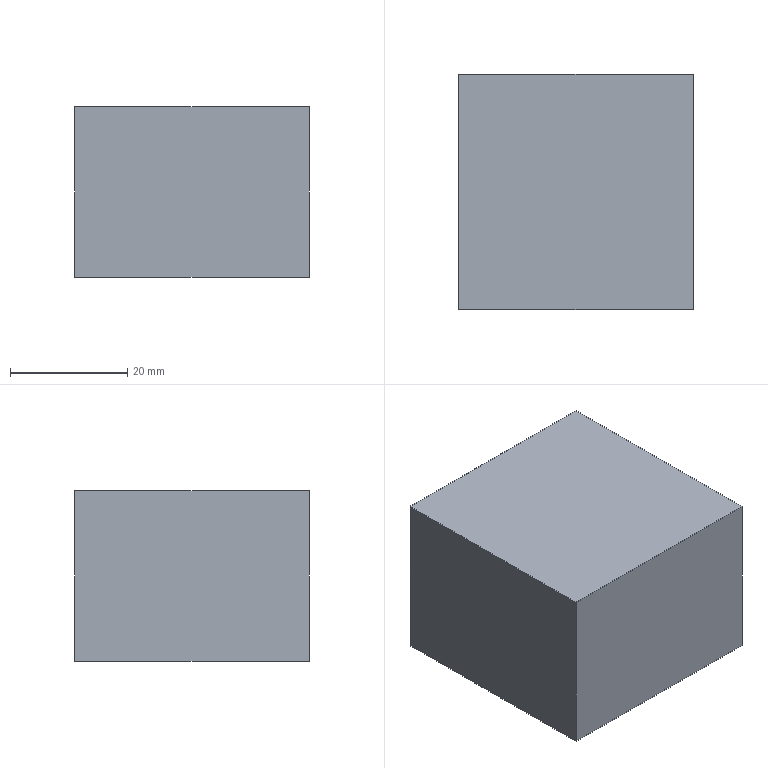Part | SolidWorks | features BaseBody 1 | 1 solid | 6 faces | box 40 x 40 x 29 mm | volume 46400 mm3 | plane 6
STEP:
#1=CARTESIAN_POINT('',(359.672,1637.809,-1184.57));
#2=VERTEX_POINT('',#1);
#3=CARTESIAN_POINT('',(319.672,1637.809,-1184.57));
#4=VERTEX_POINT('',#3);
#5=CARTESIAN_POINT('',(339.672,1637.809,-1184.57));
#6=DIRECTION('',(-1.,0.,0.));
#7=VECTOR('',#6,1000.);
#8=LINE('',#5,#7);
#9=EDGE_CURVE('',#2,#4,#8,.T.);
#10=ORIENTED_EDGE('',*,*,#9,.F.);
#11=CARTESIAN_POINT('',(359.672,1597.809,-1184.57));
#12=VERTEX_POINT('',#11);
#13=CARTESIAN_POINT('',(359.672,1617.809,-1184.57));
#14=DIRECTION('',(0.,1.,0.));
#15=VECTOR('',#14,1000.);
#16=LINE('',#13,#15);
#17=EDGE_CURVE('',#12,#2,#16,.T.);
#18=ORIENTED_EDGE('',*,*,#17,.F.);
#19=CARTESIAN_POINT('',(319.672,1597.809,-1184.57));
#20=VERTEX_POINT('',#19);
#21=CARTESIAN_POINT('',(339.672,1597.809,-1184.57));
#22=DIRECTION('',(1.,0.,0.));
#23=VECTOR('',#22,1000.);
#24=LINE('',#21,#23);
#25=EDGE_CURVE('',#20,#12,#24,.T.);
#26=ORIENTED_EDGE('',*,*,#25,.F.);
#27=CARTESIAN_POINT('',(319.672,1617.809,-1184.57));
#28=DIRECTION('',(0.,-1.,0.));
#29=VECTOR('',#28,1000.);
#30=LINE('',#27,#29);
#31=EDGE_CURVE('',#4,#20,#30,.T.);
#32=ORIENTED_EDGE('',*,*,#31,.F.);
#33=EDGE_LOOP('',(#10,#18,#26,#32));
#34=FACE_OUTER_BOUND('',#33,.T.);
#35=CARTESIAN_POINT('',(339.672,1617.809,-1184.57));
#36=DIRECTION('',(0.,0.,1.));
#37=DIRECTION('',(1.,0.,0.));
#38=AXIS2_PLACEMENT_3D('',#35,#36,#37);
#39=PLANE('',#38);
#40=ADVANCED_FACE('',(#34),#39,.F.);
#41=CARTESIAN_POINT('',(319.672,1637.809,-1155.57));
#42=VERTEX_POINT('',#41);
#43=CARTESIAN_POINT('',(319.672,1597.809,-1155.57));
#44=VERTEX_POINT('',#43);
#45=CARTESIAN_POINT('',(319.672,1637.809,-1155.57));
#46=DIRECTION('',(0.,-1.,0.));
#47=VECTOR('',#46,1000.);
#48=LINE('',#45,#47);
#49=EDGE_CURVE('',#42,#44,#48,.T.);
#50=ORIENTED_EDGE('',*,*,#49,.F.);
#51=CARTESIAN_POINT('',(319.672,1637.809,-1155.57));
#52=DIRECTION('',(0.,0.,1.));
#53=VECTOR('',#52,1000.);
#54=LINE('',#51,#53);
#55=EDGE_CURVE('',#4,#42,#54,.T.);
#56=ORIENTED_EDGE('',*,*,#55,.F.);
#57=ORIENTED_EDGE('',*,*,#31,.T.);
#58=CARTESIAN_POINT('',(319.672,1597.809,-1155.57));
#59=DIRECTION('',(0.,0.,-1.));
#60=VECTOR('',#59,1000.);
#61=LINE('',#58,#60);
#62=EDGE_CURVE('',#44,#20,#61,.T.);
#63=ORIENTED_EDGE('',*,*,#62,.F.);
#64=EDGE_LOOP('',(#50,#56,#57,#63));
#65=FACE_OUTER_BOUND('',#64,.T.);
#66=CARTESIAN_POINT('',(319.672,1637.809,-1155.57));
#67=DIRECTION('',(1.,0.,0.));
#68=DIRECTION('',(0.,0.,-1.));
#69=AXIS2_PLACEMENT_3D('',#66,#67,#68);
#70=PLANE('',#69);
#71=ADVANCED_FACE('',(#65),#70,.F.);
#72=CARTESIAN_POINT('',(359.672,1637.809,-1155.57));
#73=VERTEX_POINT('',#72);
#74=CARTESIAN_POINT('',(359.672,1637.809,-1155.57));
#75=DIRECTION('',(-1.,0.,0.));
#76=VECTOR('',#75,1000.);
#77=LINE('',#74,#76);
#78=EDGE_CURVE('',#73,#42,#77,.T.);
#79=ORIENTED_EDGE('',*,*,#78,.F.);
#80=CARTESIAN_POINT('',(359.672,1637.809,-1155.57));
#81=DIRECTION('',(0.,0.,1.));
#82=VECTOR('',#81,1000.);
#83=LINE('',#80,#82);
#84=EDGE_CURVE('',#2,#73,#83,.T.);
#85=ORIENTED_EDGE('',*,*,#84,.F.);
#86=ORIENTED_EDGE('',*,*,#9,.T.);
#87=ORIENTED_EDGE('',*,*,#55,.T.);
#88=EDGE_LOOP('',(#79,#85,#86,#87));
#89=FACE_OUTER_BOUND('',#88,.T.);
#90=CARTESIAN_POINT('',(359.672,1637.809,-1155.57));
#91=DIRECTION('',(0.,-1.,0.));
#92=DIRECTION('',(0.,0.,-1.));
#93=AXIS2_PLACEMENT_3D('',#90,#91,#92);
#94=PLANE('',#93);
#95=ADVANCED_FACE('',(#89),#94,.F.);
#96=CARTESIAN_POINT('',(359.672,1597.809,-1155.57));
#97=VERTEX_POINT('',#96);
#98=CARTESIAN_POINT('',(359.672,1637.809,-1155.57));
#99=DIRECTION('',(0.,1.,0.));
#100=VECTOR('',#99,1000.);
#101=LINE('',#98,#100);
#102=EDGE_CURVE('',#97,#73,#101,.T.);
#103=ORIENTED_EDGE('',*,*,#102,.F.);
#104=CARTESIAN_POINT('',(359.672,1597.809,-1155.57));
#105=DIRECTION('',(0.,0.,1.));
#106=VECTOR('',#105,1000.);
#107=LINE('',#104,#106);
#108=EDGE_CURVE('',#12,#97,#107,.T.);
#109=ORIENTED_EDGE('',*,*,#108,.F.);
#110=ORIENTED_EDGE('',*,*,#17,.T.);
#111=ORIENTED_EDGE('',*,*,#84,.T.);
#112=EDGE_LOOP('',(#103,#109,#110,#111));
#113=FACE_OUTER_BOUND('',#112,.T.);
#114=CARTESIAN_POINT('',(359.672,1637.809,-1155.57));
#115=DIRECTION('',(-1.,0.,0.));
#116=DIRECTION('',(0.,0.,1.));
#117=AXIS2_PLACEMENT_3D('',#114,#115,#116);
#118=PLANE('',#117);
#119=ADVANCED_FACE('',(#113),#118,.F.);
#120=CARTESIAN_POINT('',(359.672,1597.809,-1155.57));
#121=DIRECTION('',(1.,0.,0.));
#122=VECTOR('',#121,1000.);
#123=LINE('',#120,#122);
#124=EDGE_CURVE('',#44,#97,#123,.T.);
#125=ORIENTED_EDGE('',*,*,#124,.F.);
#126=ORIENTED_EDGE('',*,*,#62,.T.);
#127=ORIENTED_EDGE('',*,*,#25,.T.);
#128=ORIENTED_EDGE('',*,*,#108,.T.);
#129=EDGE_LOOP('',(#125,#126,#127,#128));
#130=FACE_OUTER_BOUND('',#129,.T.);
#131=CARTESIAN_POINT('',(359.672,1597.809,-1155.57));
#132=DIRECTION('',(0.,1.,0.));
#133=DIRECTION('',(0.,0.,1.));
#134=AXIS2_PLACEMENT_3D('',#131,#132,#133);
#135=PLANE('',#134);
#136=ADVANCED_FACE('',(#130),#135,.F.);
#137=ORIENTED_EDGE('',*,*,#49,.T.);
#138=ORIENTED_EDGE('',*,*,#124,.T.);
#139=ORIENTED_EDGE('',*,*,#102,.T.);
#140=ORIENTED_EDGE('',*,*,#78,.T.);
#141=EDGE_LOOP('',(#137,#138,#139,#140));
#142=FACE_OUTER_BOUND('',#141,.T.);
#143=CARTESIAN_POINT('',(339.672,1617.809,-1155.57));
#144=DIRECTION('',(0.,0.,1.));
#145=DIRECTION('',(1.,0.,0.));
#146=AXIS2_PLACEMENT_3D('',#143,#144,#145);
#147=PLANE('',#146);
#148=ADVANCED_FACE('',(#142),#147,.T.);
#149=CLOSED_SHELL('',(#40,#71,#95,#119,#136,#148));
#150=MANIFOLD_SOLID_BREP('',#149);
#151=CARTESIAN_POINT('',(0.,0.,0.));
#152=DIRECTION('',(0.,0.,1.));
#153=DIRECTION('',(1.,0.,0.));
#154=AXIS2_PLACEMENT_3D('',#151,#152,#153);
#155=(LENGTH_UNIT()NAMED_UNIT(*)SI_UNIT(.MILLI.,.METRE.));
#156=UNCERTAINTY_MEASURE_WITH_UNIT(LENGTH_MEASURE(0.00001),#155,'','');
#157=(NAMED_UNIT(*)PLANE_ANGLE_UNIT()SI_UNIT($,.RADIAN.));
#158=(NAMED_UNIT(*)SI_UNIT($,.STERADIAN.)SOLID_ANGLE_UNIT());
#159=(GEOMETRIC_REPRESENTATION_CONTEXT(3)GLOBAL_UNCERTAINTY_ASSIGNED_CONTEXT((#156))GLOBAL_UNIT_ASSIGNED_CONTEXT((#155,#157,#158))REPRESENTATION_CONTEXT('',''));
#160=ADVANCED_BREP_SHAPE_REPRESENTATION('',(#150,#154),#159);